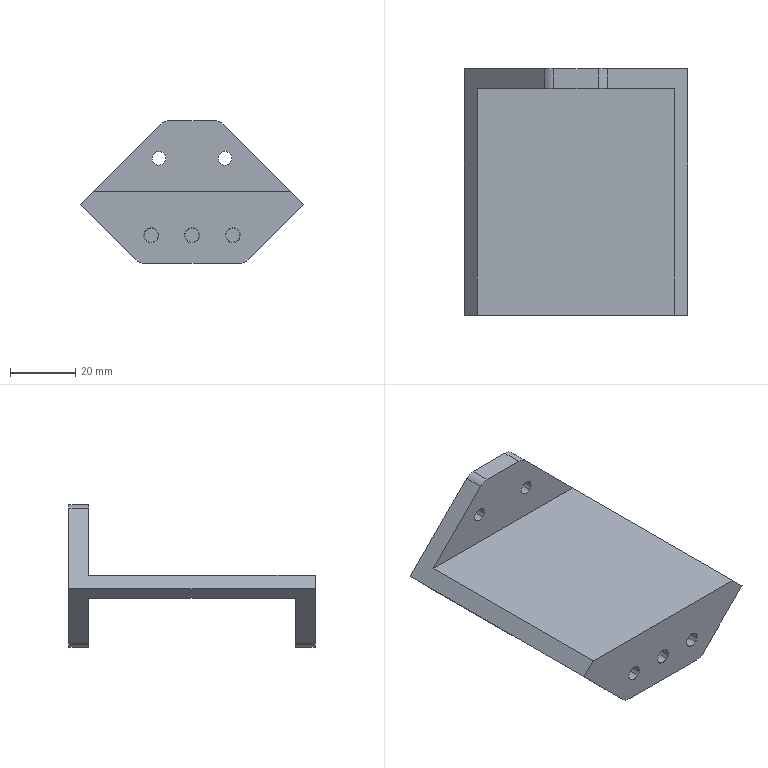NC program | NX | posted with a generic post | part box 68.307 x 75.3 x 43.668 mm
Lines 1 to 18 of 9000:
N10 G17 G21 G94 G90
(FLOOR_WALL_COPY , TOOL : D80)
N12 T19 M6
N14 G54
N16 G17 G0 G90 X86.65 Y0. B0. C0. S6500 M3
N18 G43 Z30. H19
N20 Z3.
N22 G94 G1 Z0. F1500.
N24 X81.65
N26 X-81.65
N28 X-86.65
N30 Z3.
N32 G0 Z30.
N34 M5